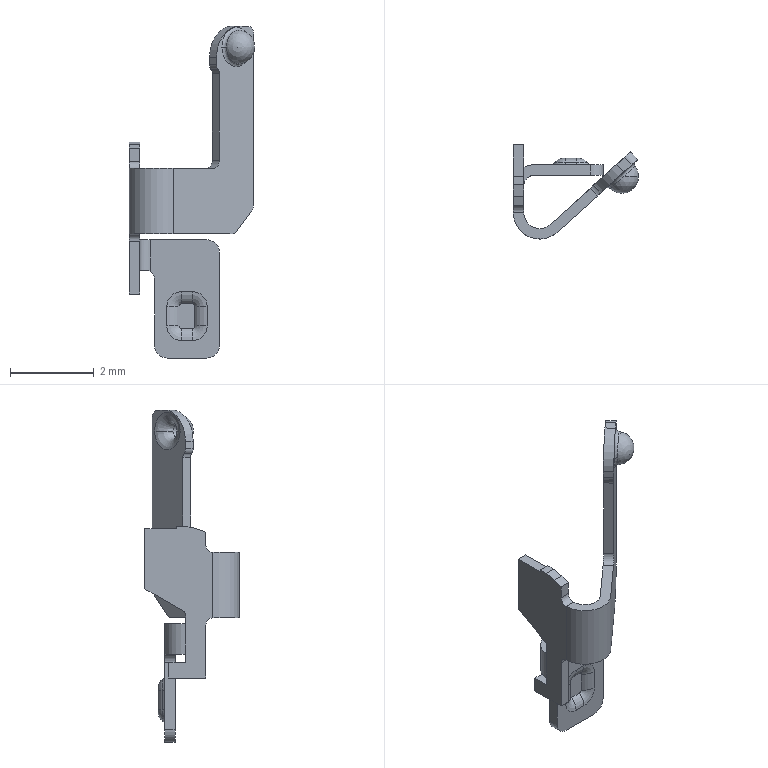Part | NX | 1 solid | 85 faces | box 2.994 x 2.25 x 7.933 mm | volume 4.65 mm3 | plane 35 | cylinder 30 | torus 16 | sphere 4 | commonest cylinder face diameters 0.5 x6 0.2 x5 0.4 x4 0.7 x4 0.6 x3 0.3 x2